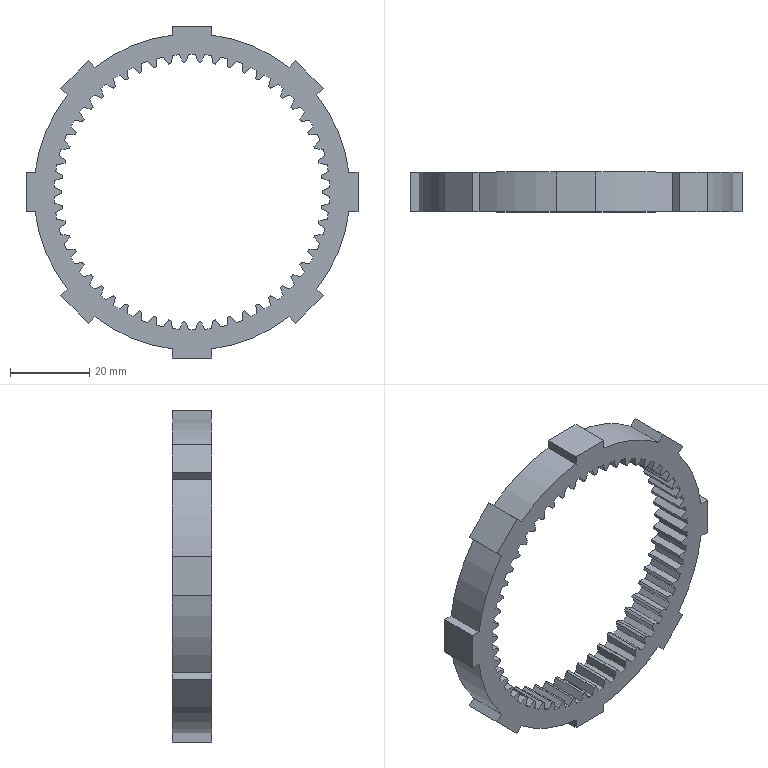Part | SolidWorks | features CirPattern 1, Extrusion 1, ICE 1 | 1 solid | 251 faces | box 84 x 10 x 84 mm | volume 15215 mm3 | cylinder 117 | spline 108 | plane 26 | commonest cylinder face diameters 69.75 x55 65.875 x54 80 x8